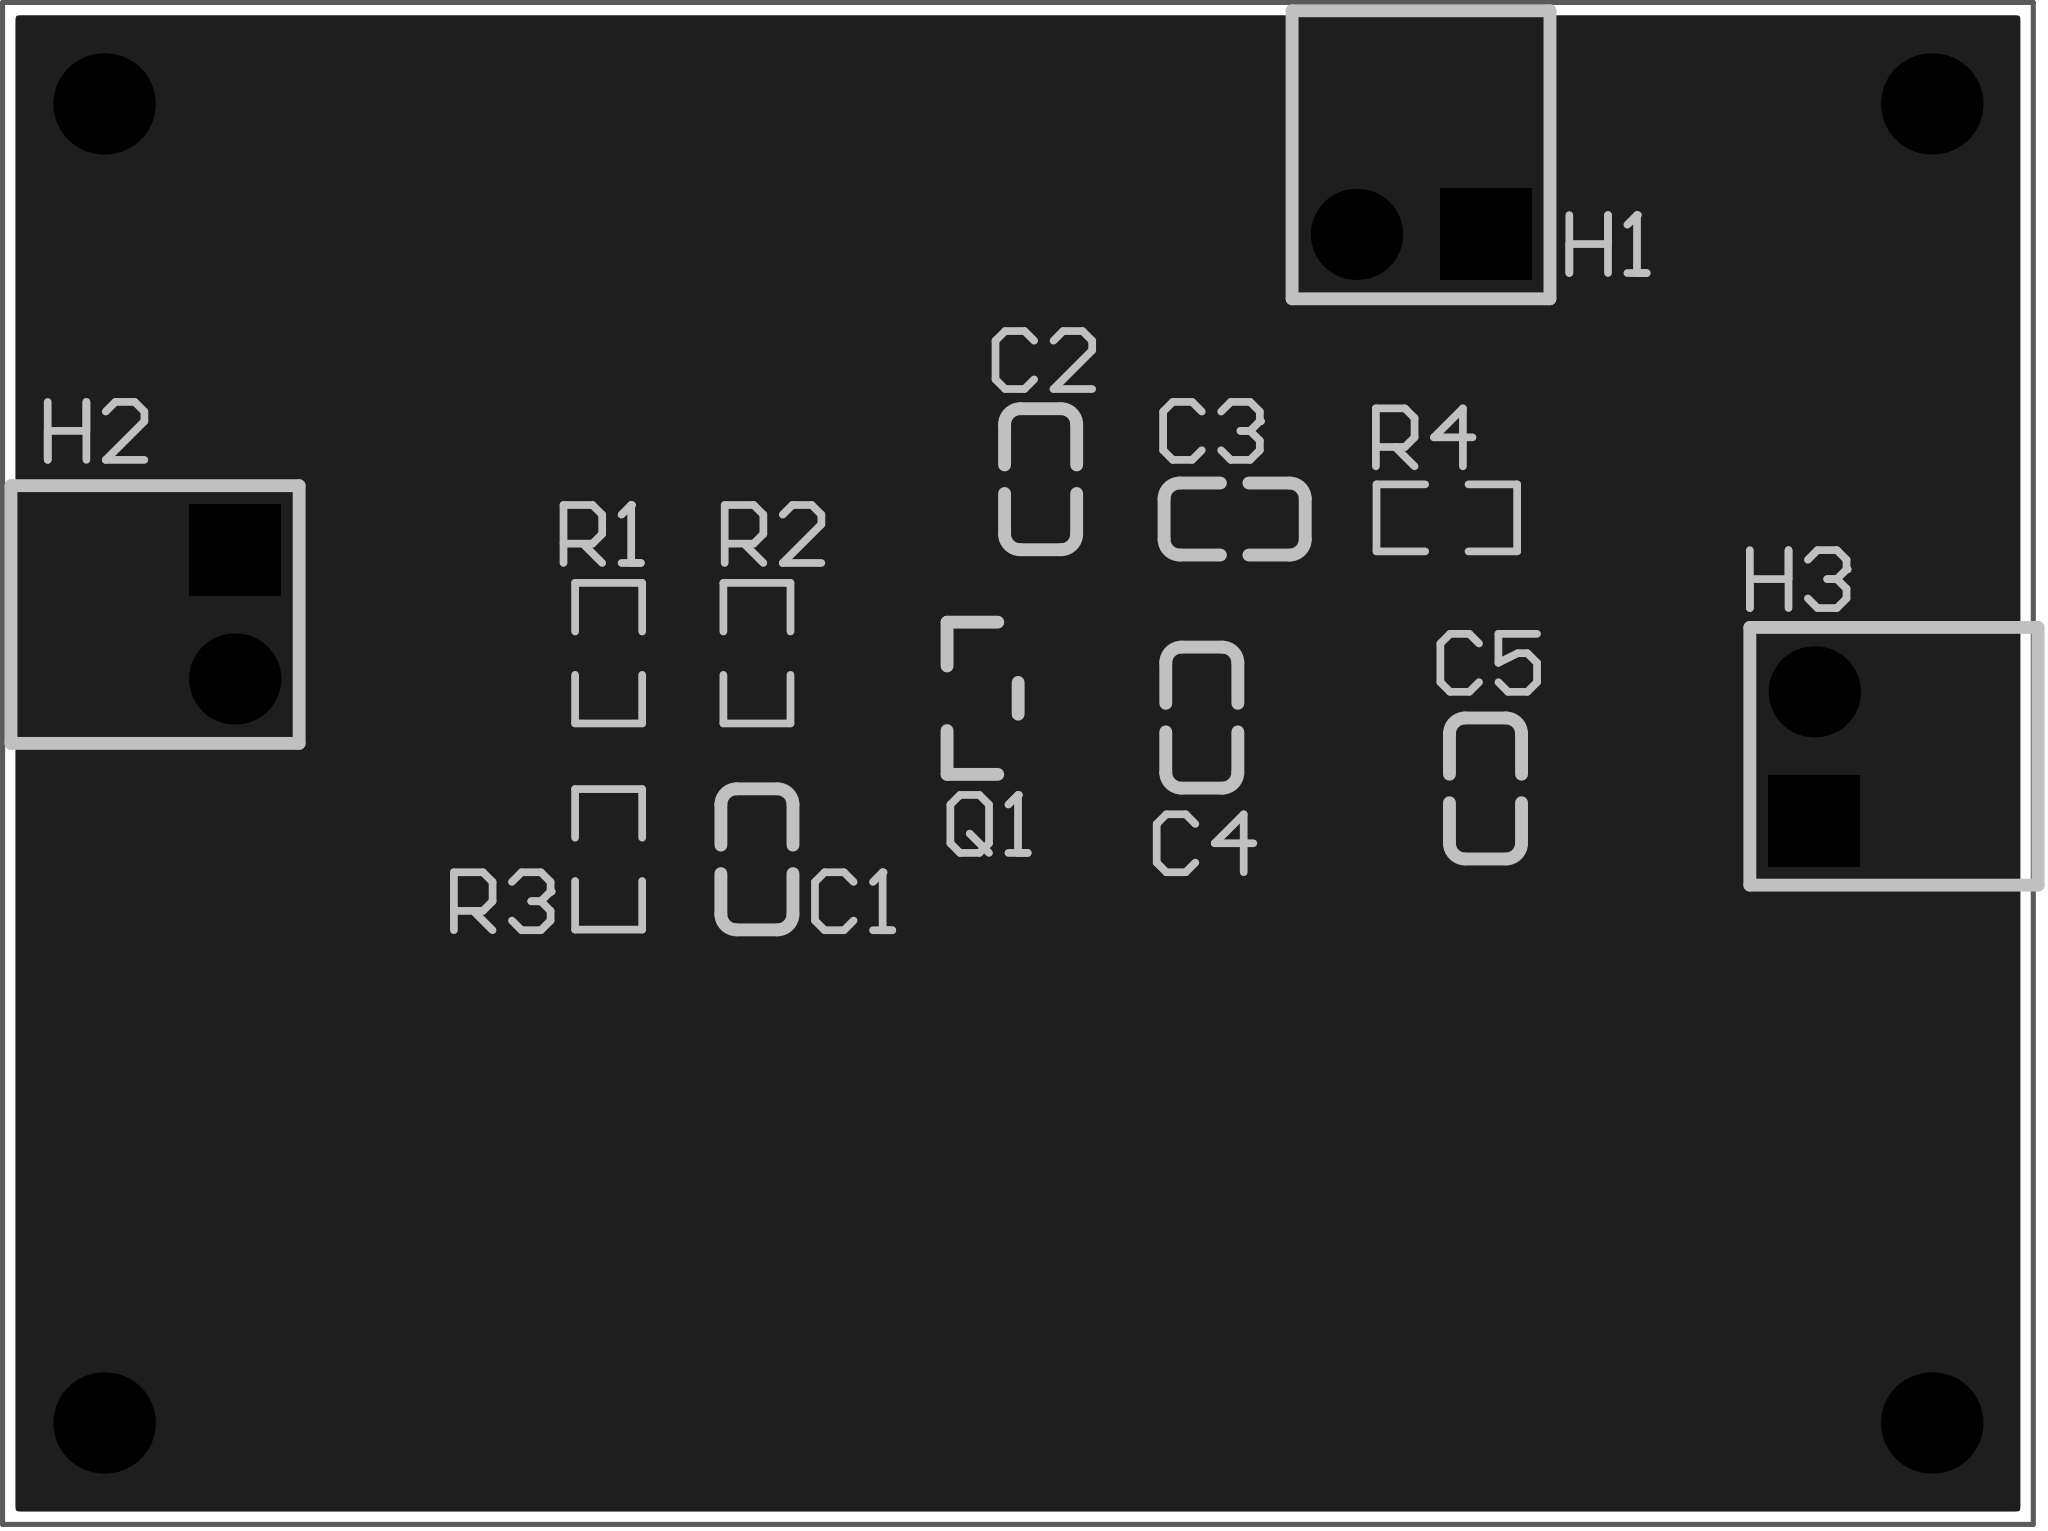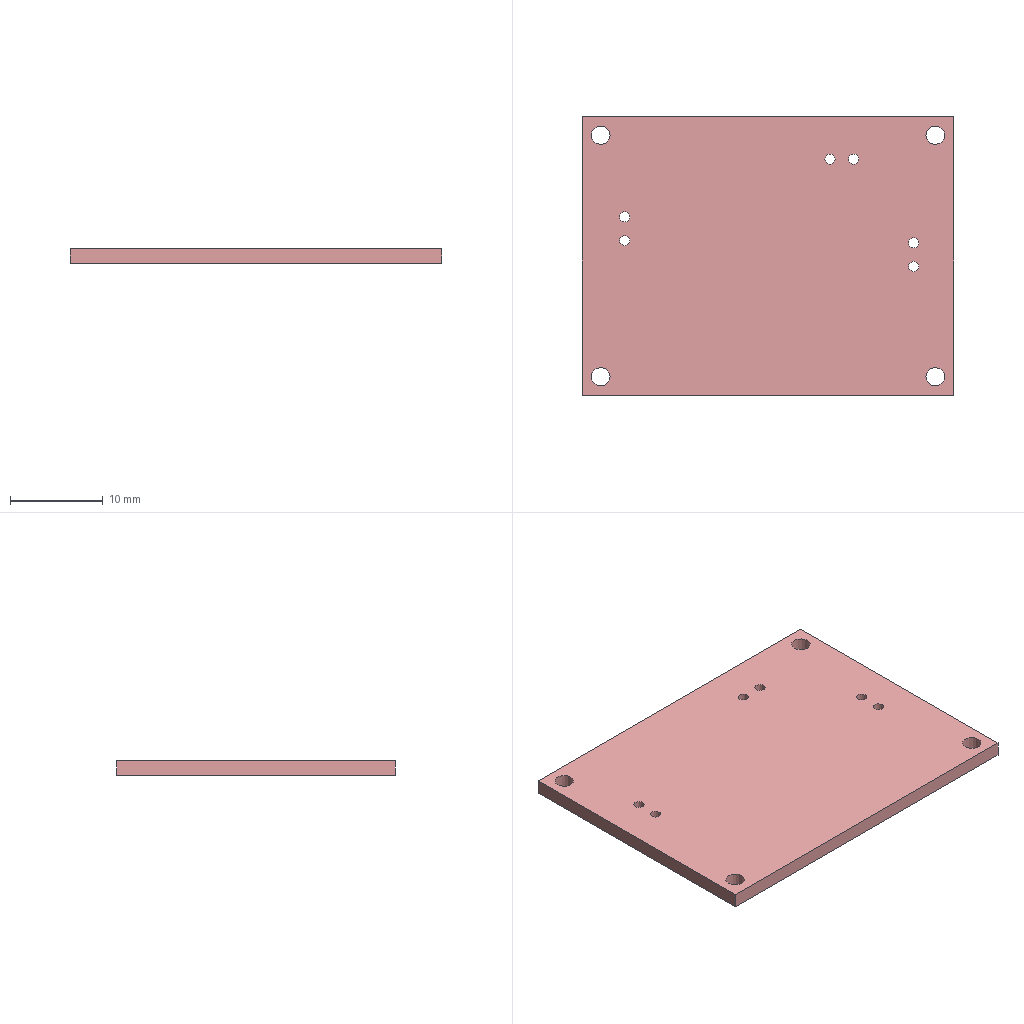Circuit board layout | Altium Designer | box 40 x 30 x 1.6 mm
Layer stack:
# Altium Designer layer stack of  (unit mm; dielectric type: 0 none, 1 core, 2 prepreg, 3 surface material)
index,name,kind,layer,copper_thickness_mm,dielectric_type,dielectric_thickness_mm,dielectric_material,dielectric_constant
0,Top Paste Mask Layer,other,,,,,,
1,Top Silkscreen Layer,other,,,,,,
2,Top Solder Mask Layer,dielectric,,,3,0.01,,3.3
3,Top Layer,copper,Top Layer,0.035,,,,
4,Dielectric1,dielectric,,,3,1.51,FR4,4.5
5,Bottom Layer,copper,Bottom Layer,0.035,,,,
6,Bottom Solder Mask Layer,dielectric,,,3,0.01,,3.3
7,Bottom Silkscreen Layer,other,,,,,,
8,Bottom Paste Mask Layer,other,,,,,,
# drill layer pairs: low layer,high layer
drill_pair,Top Layer,Bottom Layer
Part placement:
Designator,Comment,Layer,Footprint,Center-X(mm),Center-Y(mm),Rotation
H1,,TopLayer,HDR-TH_2P-P2.54-V-M-1,104.14,101.628,180
C1,20uF,TopLayer,C0603,91.059,89.309,270
C2,100nF,TopLayer,C0603,96.647,96.802,270
C3,100nF,TopLayer,C0603,100.469,96.017,0
C4,100nF,TopLayer,C0603,99.822,92.103,270
C5,20uF,TopLayer,C0603,105.41,90.706,270
H2,,TopLayer,HDR-TH_2P-P2.54-V-M-1,80.772,94.135,270
H3,,TopLayer,HDR-TH_2P-P2.54-V-M-1,111.887,91.341,90
Q1,,TopLayer,S8050_SOT-23,95.504,92.484,0
R1,1K,TopLayer,R0603,88.138,93.373,270
R2,1K,TopLayer,R0603,91.059,93.373,90
R3,4.7K,TopLayer,R0603,88.138,89.309,90
R4,10K,TopLayer,R0603,104.648,96.04,0
Pad and via stacks:
# Altium Designer via and pad stacks of  (unit mm). Each distinct definition once, with the count of objects using it.
# via: kind,start_layer,end_layer,hole_mm,diameter_mm,mode(0 simple;1 top-mid-bottom;2 full stack),diameter_per_layer,count,example_net
# pad: kind,layer,hole_mm,hole_type(0 round;1 square;2 slot),plating,top_size,top_shape(1 round;2 rect;3 octagon;9 rounded rect),mid_size,bottom_size,mode,footprint,size_per_layer,count,example
pad,Multi-Layer,2,0,plated,2x2,1,2x2,2x2,0,,,4,1
pad,Multi-Layer,1.1,0,plated,1.8x1.8,1,1.8x1.8,1.8x1.8,0,HDR-TH_2P-P2.54-V-M-1,,3,H1.2
pad,Multi-Layer,1.1,0,plated,1.8x1.8,2,1.8x1.8,1.8x1.8,0,HDR-TH_2P-P2.54-V-M-1,,3,H1.1
pad,Top Layer,0,0,plated,0.8x0.9,2,0.8x0.9,0.8x0.9,0,C0603,,10,C1.2
pad,Top Layer,0,0,plated,1x0.8,2,1x0.8,1x0.8,0,S8050_SOT-23,,3,Q1.2
pad,Top Layer,0,0,plated,0.8065x0.864,2,0.8065x0.864,0.8065x0.864,0,R0603,,8,R1.2
Copper pours:
name,layer,net,type(0 solid;1 hatched;2 none)
Top Layer-GND,Top Layer,GND,0
Bottom Layer-GND,Bottom Layer,GND,0
Design rules, without the lines most boards share:
# Altium Designer design rules of  (exported by Altium Designer, unit mm)
# columns: name | kind | enabled | priority | scope1 | scope2 | descriptor | typed fields (field=value)
creepage | 65 | enabled | 1 | All | All | Creepage Distance Constraint =(0mil) (All),(All) |